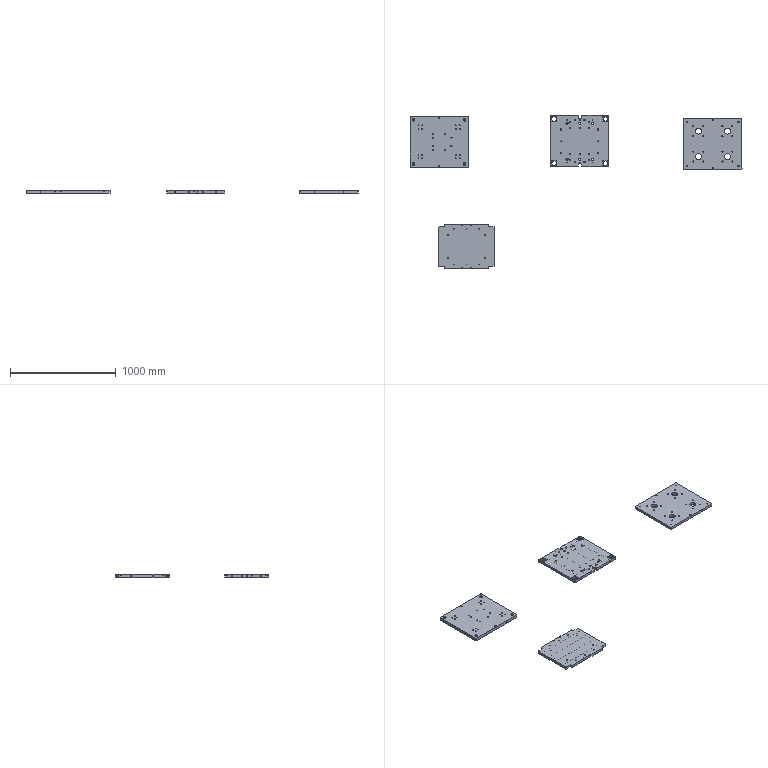NC program | Mastercam | posted with a generic post | part box 3140 x 1452 x 30 mm
Lines 1914 to 2558 of 6493:
N9180 T5 M6
N9190 G0 G90 G17 G54 X-192.57 Y156. A0. S6000 M3
N9200 G43 H5 Z50. M8
N9210 Z1.2
N9220 G1 Z.2 F600.
N9230 G3 X-194.5 Y157.93 Z.1 I-1.93 J0. F2000.
N9240 X-196.43 Y156. Z0. I0. J-1.93
N9250 X-194.5 Y154.07 Z-.1 I1.93 J0.
N9260 X-192.57 Y156. Z-.2 I0. J1.93
N9270 X-194.5 Y157.93 Z-.3 I-1.93 J0.
N9280 X-196.43 Y156. Z-.4 I0. J-1.93
N9290 X-194.5 Y154.07 Z-.5 I1.93 J0.
N9300 X-192.57 Y156. Z-.6 I0. J1.93
N9310 X-194.5 Y157.93 Z-.7 I-1.93 J0.
N9320 X-196.43 Y156. Z-.8 I0. J-1.93
N9330 X-194.5 Y154.07 Z-.9 I1.93 J0.
N9340 X-192.57 Y156. Z-1. I0. J1.93
N9350 X-194.5 Y157.93 Z-1.1 I-1.93 J0.
N9360 X-196.43 Y156. Z-1.2 I0. J-1.93
N9370 X-194.5 Y154.07 Z-1.3 I1.93 J0.
N9380 X-192.57 Y156. Z-1.4 I0. J1.93
N9390 X-194.5 Y157.93 Z-1.5 I-1.93 J0.
N9400 X-196.43 Y156. Z-1.6 I0. J-1.93
N9410 X-194.5 Y154.07 Z-1.7 I1.93 J0.
N9420 X-192.57 Y156. Z-1.8 I0. J1.93
N9430 X-194.5 Y157.93 Z-1.9 I-1.93 J0.
N9440 X-196.43 Y156. Z-2. I0. J-1.93
N9450 X-194.5 Y154.07 Z-2.1 I1.93 J0.
N9460 X-192.57 Y156. Z-2.2 I0. J1.93
N9470 X-194.5 Y157.93 Z-2.3 I-1.93 J0.
N9480 X-196.43 Y156. Z-2.4 I0. J-1.93
N9490 X-194.5 Y154.07 Z-2.5 I1.93 J0.
N9500 X-192.57 Y156. Z-2.6 I0. J1.93
N9510 X-194.5 Y157.93 Z-2.7 I-1.93 J0.
N9520 X-196.43 Y156. Z-2.8 I0. J-1.93
N9530 X-194.5 Y154.07 Z-2.9 I1.93 J0.
N9540 X-192.57 Y156. Z-3. I0. J1.93
N9550 X-194.5 Y157.93 Z-3.1 I-1.93 J0.
N9560 X-196.43 Y156. Z-3.2 I0. J-1.93
N9570 X-194.5 Y154.07 Z-3.3 I1.93 J0.
N9580 X-192.57 Y156. Z-3.4 I0. J1.93
N9590 X-194.5 Y157.93 Z-3.5 I-1.93 J0.
N9600 X-196.43 Y156. Z-3.6 I0. J-1.93
N9610 X-194.5 Y154.07 Z-3.7 I1.93 J0.
N9620 X-192.57 Y156. Z-3.8 I0. J1.93
N9630 X-194.5 Y157.93 Z-3.9 I-1.93 J0.
N9640 X-196.43 Y156. Z-4. I0. J-1.93
N9650 X-194.5 Y154.07 Z-4.1 I1.93 J0.
N9660 X-192.57 Y156. Z-4.2 I0. J1.93
N9670 X-194.5 Y157.93 Z-4.3 I-1.93 J0.
N9680 X-196.43 Y156. Z-4.4 I0. J-1.93
N9690 X-194.5 Y154.07 Z-4.5 I1.93 J0.
N9700 X-192.57 Y156. Z-4.6 I0. J1.93
N9710 X-194.5 Y157.93 Z-4.7 I-1.93 J0.
N9720 X-196.43 Y156. Z-4.8 I0. J-1.93
N9730 X-194.5 Y154.07 Z-4.9 I1.93 J0.
N9740 X-192.57 Y156. Z-5. I0. J1.93
N9750 X-194.5 Y157.93 Z-5.1 I-1.93 J0.
N9760 X-196.43 Y156. Z-5.2 I0. J-1.93
N9770 X-194.5 Y154.07 Z-5.3 I1.93 J0.
N9780 X-192.57 Y156. Z-5.4 I0. J1.93
N9790 X-194.5 Y157.93 Z-5.5 I-1.93 J0.
N9800 X-196.43 Y156. Z-5.6 I0. J-1.93
N9810 X-194.5 Y154.07 Z-5.7 I1.93 J0.
N9820 X-192.57 Y156. Z-5.8 I0. J1.93
N9830 X-194.5 Y157.93 Z-5.9 I-1.93 J0.
N9840 X-196.43 Y156. Z-6. I0. J-1.93
N9850 X-194.5 Y154.07 Z-6.1 I1.93 J0.
N9860 X-192.57 Y156. Z-6.2 I0. J1.93
N9870 X-194.5 Y157.93 Z-6.3 I-1.93 J0.
N9880 X-196.43 Y156. Z-6.4 I0. J-1.93
N9890 X-194.5 Y154.07 Z-6.5 I1.93 J0.
N9900 X-192.57 Y156. Z-6.6 I0. J1.93
N9910 X-194.5 Y157.93 Z-6.7 I-1.93 J0.
N9920 X-196.43 Y156. Z-6.8 I0. J-1.93
N9930 X-194.5 Y154.07 Z-6.9 I1.93 J0.
N9940 X-192.57 Y156. Z-7. I0. J1.93
N9950 X-194.5 Y157.93 Z-7.1 I-1.93 J0.
N9960 X-196.43 Y156. Z-7.2 I0. J-1.93
N9970 X-194.5 Y154.07 Z-7.3 I1.93 J0.
N9980 X-192.57 Y156. Z-7.4 I0. J1.93
N9990 X-194.5 Y157.93 Z-7.5 I-1.93 J0.
N100 X-196.43 Y156. Z-7.6 I0. J-1.93
N110 X-194.5 Y154.07 Z-7.7 I1.93 J0.
N120 X-192.57 Y156. Z-7.8 I0. J1.93
N130 X-194.5 Y157.93 Z-7.9 I-1.93 J0.
N140 X-196.43 Y156. Z-8. I0. J-1.93
N150 X-194.5 Y154.07 Z-8.1 I1.93 J0.
N160 X-192.57 Y156. Z-8.2 I0. J1.93
N170 X-194.5 Y157.93 Z-8.3 I-1.93 J0.
N180 X-196.43 Y156. Z-8.4 I0. J-1.93
N190 X-194.5 Y154.07 Z-8.5 I1.93 J0.
N200 X-192.57 Y156. Z-8.6 I0. J1.93
N210 X-194.5 Y157.93 Z-8.7 I-1.93 J0.
N220 X-196.43 Y156. Z-8.8 I0. J-1.93
N230 X-194.5 Y154.07 Z-8.9 I1.93 J0.
N240 X-192.57 Y156. Z-9. I0. J1.93
N250 X-194.5 Y157.93 Z-9.1 I-1.93 J0.
N260 X-196.43 Y156. Z-9.2 I0. J-1.93
N270 X-194.5 Y154.07 Z-9.3 I1.93 J0.
N280 X-192.57 Y156. Z-9.4 I0. J1.93
N290 X-194.5 Y157.93 Z-9.5 I-1.93 J0.
N300 X-196.43 Y156. Z-9.6 I0. J-1.93
N310 X-194.5 Y154.07 Z-9.7 I1.93 J0.
N320 X-192.57 Y156. Z-9.8 I0. J1.93
N330 X-194.5 Y157.93 Z-9.9 I-1.93 J0.
N340 X-196.43 Y156. Z-10. I0. J-1.93
N350 X-194.5 Y154.07 Z-10.1 I1.93 J0.
N360 X-192.57 Y156. Z-10.2 I0. J1.93
N370 X-194.5 Y157.93 Z-10.3 I-1.93 J0.
N380 X-196.43 Y156. Z-10.4 I0. J-1.93
N390 X-194.5 Y154.07 Z-10.5 I1.93 J0.
N400 X-192.57 Y156. Z-10.6 I0. J1.93
N410 X-194.5 Y157.93 Z-10.7 I-1.93 J0.
N420 X-196.43 Y156. Z-10.8 I0. J-1.93
N430 X-194.5 Y154.07 Z-10.9 I1.93 J0.
N440 X-192.57 Y156. Z-11. I0. J1.93
N450 X-194.5 Y157.93 Z-11.1 I-1.93 J0.
N460 X-196.43 Y156. Z-11.2 I0. J-1.93
N470 X-194.5 Y154.07 Z-11.3 I1.93 J0.
N480 X-192.57 Y156. Z-11.4 I0. J1.93
N490 X-194.5 Y157.93 Z-11.5 I-1.93 J0.
N500 X-196.43 Y156. Z-11.6 I0. J-1.93
N510 X-194.5 Y154.07 Z-11.7 I1.93 J0.
N520 X-192.57 Y156. Z-11.8 I0. J1.93
N530 X-194.5 Y157.93 Z-11.9 I-1.93 J0.
N540 X-196.43 Y156. Z-12. I0. J-1.93
N550 X-194.5 Y154.07 Z-12.1 I1.93 J0.
N560 X-192.57 Y156. Z-12.2 I0. J1.93
N570 X-194.5 Y157.93 Z-12.3 I-1.93 J0.
N580 X-196.43 Y156. Z-12.4 I0. J-1.93
N590 X-194.5 Y154.07 Z-12.5 I1.93 J0.
N600 X-192.57 Y156. Z-12.6 I0. J1.93
N610 X-194.5 Y157.93 Z-12.7 I-1.93 J0.
N620 X-196.43 Y156. Z-12.8 I0. J-1.93
N630 X-194.5 Y154.07 Z-12.9 I1.93 J0.
N640 X-192.57 Y156. Z-13. I0. J1.93
N650 X-194.5 Y157.93 Z-13.1 I-1.93 J0.
N660 X-196.43 Y156. Z-13.2 I0. J-1.93
N670 X-194.5 Y154.07 Z-13.3 I1.93 J0.
N680 X-192.57 Y156. Z-13.4 I0. J1.93
N690 X-194.5 Y157.93 Z-13.5 I-1.93 J0.
N700 X-196.43 Y156. Z-13.6 I0. J-1.93
N710 X-194.5 Y154.07 Z-13.7 I1.93 J0.
N720 X-192.57 Y156. Z-13.8 I0. J1.93
N730 X-194.5 Y157.93 Z-13.9 I-1.93 J0.
N740 X-195.865 Y157.365 Z-13.95 I0. J-1.93
N750 X-196.43 Y156. I1.365 J-1.365
N760 X-194.5 Y154.07 I1.93 J0.
N770 X-192.57 Y156. I0. J1.93
N780 X-194.5 Y157.93 I-1.93 J0.
N790 X-196.169 Y156.97 I0. J-1.93
N800 G0 Z50.
N810 X-192.57 Y124.
N820 Z1.2
N830 G1 Z.2 F600.
N840 G3 X-194.5 Y125.93 Z.1 I-1.93 J0. F2000.
N850 X-196.43 Y124. Z0. I0. J-1.93
N860 X-194.5 Y122.07 Z-.1 I1.93 J0.
N870 X-192.57 Y124. Z-.2 I0. J1.93
N880 X-194.5 Y125.93 Z-.3 I-1.93 J0.
N890 X-196.43 Y124. Z-.4 I0. J-1.93
N900 X-194.5 Y122.07 Z-.5 I1.93 J0.
N910 X-192.57 Y124. Z-.6 I0. J1.93
N920 X-194.5 Y125.93 Z-.7 I-1.93 J0.
N930 X-196.43 Y124. Z-.8 I0. J-1.93
N940 X-194.5 Y122.07 Z-.9 I1.93 J0.
N950 X-192.57 Y124. Z-1. I0. J1.93
N960 X-194.5 Y125.93 Z-1.1 I-1.93 J0.
N970 X-196.43 Y124. Z-1.2 I0. J-1.93
N980 X-194.5 Y122.07 Z-1.3 I1.93 J0.
N990 X-192.57 Y124. Z-1.4 I0. J1.93
N1000 X-194.5 Y125.93 Z-1.5 I-1.93 J0.
N1010 X-196.43 Y124. Z-1.6 I0. J-1.93
N1020 X-194.5 Y122.07 Z-1.7 I1.93 J0.
N1030 X-192.57 Y124. Z-1.8 I0. J1.93
N1040 X-194.5 Y125.93 Z-1.9 I-1.93 J0.
N1050 X-196.43 Y124. Z-2. I0. J-1.93
N1060 X-194.5 Y122.07 Z-2.1 I1.93 J0.
N1070 X-192.57 Y124. Z-2.2 I0. J1.93
N1080 X-194.5 Y125.93 Z-2.3 I-1.93 J0.
N1090 X-196.43 Y124. Z-2.4 I0. J-1.93
N1100 X-194.5 Y122.07 Z-2.5 I1.93 J0.
N1110 X-192.57 Y124. Z-2.6 I0. J1.93
N1120 X-194.5 Y125.93 Z-2.7 I-1.93 J0.
N1130 X-196.43 Y124. Z-2.8 I0. J-1.93
N1140 X-194.5 Y122.07 Z-2.9 I1.93 J0.
N1150 X-192.57 Y124. Z-3. I0. J1.93
N1160 X-194.5 Y125.93 Z-3.1 I-1.93 J0.
N1170 X-196.43 Y124. Z-3.2 I0. J-1.93
N1180 X-194.5 Y122.07 Z-3.3 I1.93 J0.
N1190 X-192.57 Y124. Z-3.4 I0. J1.93
N1200 X-194.5 Y125.93 Z-3.5 I-1.93 J0.
N1210 X-196.43 Y124. Z-3.6 I0. J-1.93
N1220 X-194.5 Y122.07 Z-3.7 I1.93 J0.
N1230 X-192.57 Y124. Z-3.8 I0. J1.93
N1240 X-194.5 Y125.93 Z-3.9 I-1.93 J0.
N1250 X-196.43 Y124. Z-4. I0. J-1.93
N1260 X-194.5 Y122.07 Z-4.1 I1.93 J0.
N1270 X-192.57 Y124. Z-4.2 I0. J1.93
N1280 X-194.5 Y125.93 Z-4.3 I-1.93 J0.
N1290 X-196.43 Y124. Z-4.4 I0. J-1.93
N1300 X-194.5 Y122.07 Z-4.5 I1.93 J0.
N1310 X-192.57 Y124. Z-4.6 I0. J1.93
N1320 X-194.5 Y125.93 Z-4.7 I-1.93 J0.
N1330 X-196.43 Y124. Z-4.8 I0. J-1.93
N1340 X-194.5 Y122.07 Z-4.9 I1.93 J0.
N1350 X-192.57 Y124. Z-5. I0. J1.93
N1360 X-194.5 Y125.93 Z-5.1 I-1.93 J0.
N1370 X-196.43 Y124. Z-5.2 I0. J-1.93
N1380 X-194.5 Y122.07 Z-5.3 I1.93 J0.
N1390 X-192.57 Y124. Z-5.4 I0. J1.93
N1400 X-194.5 Y125.93 Z-5.5 I-1.93 J0.
N1410 X-196.43 Y124. Z-5.6 I0. J-1.93
N1420 X-194.5 Y122.07 Z-5.7 I1.93 J0.
N1430 X-192.57 Y124. Z-5.8 I0. J1.93
N1440 X-194.5 Y125.93 Z-5.9 I-1.93 J0.
N1450 X-196.43 Y124. Z-6. I0. J-1.93
N1460 X-194.5 Y122.07 Z-6.1 I1.93 J0.
N1470 X-192.57 Y124. Z-6.2 I0. J1.93
N1480 X-194.5 Y125.93 Z-6.3 I-1.93 J0.
N1490 X-196.43 Y124. Z-6.4 I0. J-1.93
N1500 X-194.5 Y122.07 Z-6.5 I1.93 J0.
N1510 X-192.57 Y124. Z-6.6 I0. J1.93
N1520 X-194.5 Y125.93 Z-6.7 I-1.93 J0.
N1530 X-196.43 Y124. Z-6.8 I0. J-1.93
N1540 X-194.5 Y122.07 Z-6.9 I1.93 J0.
N1550 X-192.57 Y124. Z-7. I0. J1.93
N1560 X-194.5 Y125.93 Z-7.1 I-1.93 J0.
N1570 X-196.43 Y124. Z-7.2 I0. J-1.93
N1580 X-194.5 Y122.07 Z-7.3 I1.93 J0.
N1590 X-192.57 Y124. Z-7.4 I0. J1.93
N1600 X-194.5 Y125.93 Z-7.5 I-1.93 J0.
N1610 X-196.43 Y124. Z-7.6 I0. J-1.93
N1620 X-194.5 Y122.07 Z-7.7 I1.93 J0.
N1630 X-192.57 Y124. Z-7.8 I0. J1.93
N1640 X-194.5 Y125.93 Z-7.9 I-1.93 J0.
N1650 X-196.43 Y124. Z-8. I0. J-1.93
N1660 X-194.5 Y122.07 Z-8.1 I1.93 J0.
N1670 X-192.57 Y124. Z-8.2 I0. J1.93
N1680 X-194.5 Y125.93 Z-8.3 I-1.93 J0.
N1690 X-196.43 Y124. Z-8.4 I0. J-1.93
N1700 X-194.5 Y122.07 Z-8.5 I1.93 J0.
N1710 X-192.57 Y124. Z-8.6 I0. J1.93
N1720 X-194.5 Y125.93 Z-8.7 I-1.93 J0.
N1730 X-196.43 Y124. Z-8.8 I0. J-1.93
N1740 X-194.5 Y122.07 Z-8.9 I1.93 J0.
N1750 X-192.57 Y124. Z-9. I0. J1.93
N1760 X-194.5 Y125.93 Z-9.1 I-1.93 J0.
N1770 X-196.43 Y124. Z-9.2 I0. J-1.93
N1780 X-194.5 Y122.07 Z-9.3 I1.93 J0.
N1790 X-192.57 Y124. Z-9.4 I0. J1.93
N1800 X-194.5 Y125.93 Z-9.5 I-1.93 J0.
N1810 X-196.43 Y124. Z-9.6 I0. J-1.93
N1820 X-194.5 Y122.07 Z-9.7 I1.93 J0.
N1830 X-192.57 Y124. Z-9.8 I0. J1.93
N1840 X-194.5 Y125.93 Z-9.9 I-1.93 J0.
N1850 X-196.43 Y124. Z-10. I0. J-1.93
N1860 X-194.5 Y122.07 Z-10.1 I1.93 J0.
N1870 X-192.57 Y124. Z-10.2 I0. J1.93
N1880 X-194.5 Y125.93 Z-10.3 I-1.93 J0.
N1890 X-196.43 Y124. Z-10.4 I0. J-1.93
N1900 X-194.5 Y122.07 Z-10.5 I1.93 J0.
N1910 X-192.57 Y124. Z-10.6 I0. J1.93
N1920 X-194.5 Y125.93 Z-10.7 I-1.93 J0.
N1930 X-196.43 Y124. Z-10.8 I0. J-1.93
N1940 X-194.5 Y122.07 Z-10.9 I1.93 J0.
N1950 X-192.57 Y124. Z-11. I0. J1.93
N1960 X-194.5 Y125.93 Z-11.1 I-1.93 J0.
N1970 X-196.43 Y124. Z-11.2 I0. J-1.93
N1980 X-194.5 Y122.07 Z-11.3 I1.93 J0.
N1990 X-192.57 Y124. Z-11.4 I0. J1.93
N2000 X-194.5 Y125.93 Z-11.5 I-1.93 J0.
N2010 X-196.43 Y124. Z-11.6 I0. J-1.93
N2020 X-194.5 Y122.07 Z-11.7 I1.93 J0.
N2030 X-192.57 Y124. Z-11.8 I0. J1.93
N2040 X-194.5 Y125.93 Z-11.9 I-1.93 J0.
N2050 X-196.43 Y124. Z-12. I0. J-1.93
N2060 X-194.5 Y122.07 Z-12.1 I1.93 J0.
N2070 X-192.57 Y124. Z-12.2 I0. J1.93
N2080 X-194.5 Y125.93 Z-12.3 I-1.93 J0.
N2090 X-196.43 Y124. Z-12.4 I0. J-1.93
N2100 X-194.5 Y122.07 Z-12.5 I1.93 J0.
N2110 X-192.57 Y124. Z-12.6 I0. J1.93
N2120 X-194.5 Y125.93 Z-12.7 I-1.93 J0.
N2130 X-196.43 Y124. Z-12.8 I0. J-1.93
N2140 X-194.5 Y122.07 Z-12.9 I1.93 J0.
N2150 X-192.57 Y124. Z-13. I0. J1.93
N2160 X-194.5 Y125.93 Z-13.1 I-1.93 J0.
N2170 X-196.43 Y124. Z-13.2 I0. J-1.93
N2180 X-194.5 Y122.07 Z-13.3 I1.93 J0.
N2190 X-192.57 Y124. Z-13.4 I0. J1.93
N2200 X-194.5 Y125.93 Z-13.5 I-1.93 J0.
N2210 X-196.43 Y124. Z-13.6 I0. J-1.93
N2220 X-194.5 Y122.07 Z-13.7 I1.93 J0.
N2230 X-192.57 Y124. Z-13.8 I0. J1.93
N2240 X-194.5 Y125.93 Z-13.9 I-1.93 J0.
N2250 X-195.865 Y125.365 Z-13.95 I0. J-1.93
N2260 X-196.43 Y124. I1.365 J-1.365
N2270 X-194.5 Y122.07 I1.93 J0.
N2280 X-192.57 Y124. I0. J1.93
N2290 X-194.5 Y125.93 I-1.93 J0.
N2300 X-196.169 Y124.97 I0. J-1.93
N2310 G0 Z50.
N2320 X-156.57 Y156.
N2330 Z1.2
N2340 G1 Z.2 F600.
N2350 G3 X-158.5 Y157.93 Z.1 I-1.93 J0. F2000.
N2360 X-160.43 Y156. Z0. I0. J-1.93
N2370 X-158.5 Y154.07 Z-.1 I1.93 J0.
N2380 X-156.57 Y156. Z-.2 I0. J1.93
N2390 X-158.5 Y157.93 Z-.3 I-1.93 J0.
N2400 X-160.43 Y156. Z-.4 I0. J-1.93
N2410 X-158.5 Y154.07 Z-.5 I1.93 J0.
N2420 X-156.57 Y156. Z-.6 I0. J1.93
N2430 X-158.5 Y157.93 Z-.7 I-1.93 J0.
N2440 X-160.43 Y156. Z-.8 I0. J-1.93
N2450 X-158.5 Y154.07 Z-.9 I1.93 J0.
N2460 X-156.57 Y156. Z-1. I0. J1.93
N2470 X-158.5 Y157.93 Z-1.1 I-1.93 J0.
N2480 X-160.43 Y156. Z-1.2 I0. J-1.93
N2490 X-158.5 Y154.07 Z-1.3 I1.93 J0.
N2500 X-156.57 Y156. Z-1.4 I0. J1.93
N2510 X-158.5 Y157.93 Z-1.5 I-1.93 J0.
N2520 X-160.43 Y156. Z-1.6 I0. J-1.93
N2530 X-158.5 Y154.07 Z-1.7 I1.93 J0.
N2540 X-156.57 Y156. Z-1.8 I0. J1.93
N2550 X-158.5 Y157.93 Z-1.9 I-1.93 J0.
N2560 X-160.43 Y156. Z-2. I0. J-1.93
N2570 X-158.5 Y154.07 Z-2.1 I1.93 J0.
N2580 X-156.57 Y156. Z-2.2 I0. J1.93
N2590 X-158.5 Y157.93 Z-2.3 I-1.93 J0.
N2600 X-160.43 Y156. Z-2.4 I0. J-1.93
N2610 X-158.5 Y154.07 Z-2.5 I1.93 J0.
N2620 X-156.57 Y156. Z-2.6 I0. J1.93
N2630 X-158.5 Y157.93 Z-2.7 I-1.93 J0.
N2640 X-160.43 Y156. Z-2.8 I0. J-1.93
N2650 X-158.5 Y154.07 Z-2.9 I1.93 J0.
N2660 X-156.57 Y156. Z-3. I0. J1.93
N2670 X-158.5 Y157.93 Z-3.1 I-1.93 J0.
N2680 X-160.43 Y156. Z-3.2 I0. J-1.93
N2690 X-158.5 Y154.07 Z-3.3 I1.93 J0.
N2700 X-156.57 Y156. Z-3.4 I0. J1.93
N2710 X-158.5 Y157.93 Z-3.5 I-1.93 J0.
N2720 X-160.43 Y156. Z-3.6 I0. J-1.93
N2730 X-158.5 Y154.07 Z-3.7 I1.93 J0.
N2740 X-156.57 Y156. Z-3.8 I0. J1.93
N2750 X-158.5 Y157.93 Z-3.9 I-1.93 J0.
N2760 X-160.43 Y156. Z-4. I0. J-1.93
N2770 X-158.5 Y154.07 Z-4.1 I1.93 J0.
N2780 X-156.57 Y156. Z-4.2 I0. J1.93
N2790 X-158.5 Y157.93 Z-4.3 I-1.93 J0.
N2800 X-160.43 Y156. Z-4.4 I0. J-1.93
N2810 X-158.5 Y154.07 Z-4.5 I1.93 J0.
N2820 X-156.57 Y156. Z-4.6 I0. J1.93
N2830 X-158.5 Y157.93 Z-4.7 I-1.93 J0.
N2840 X-160.43 Y156. Z-4.8 I0. J-1.93
N2850 X-158.5 Y154.07 Z-4.9 I1.93 J0.
N2860 X-156.57 Y156. Z-5. I0. J1.93
N2870 X-158.5 Y157.93 Z-5.1 I-1.93 J0.
N2880 X-160.43 Y156. Z-5.2 I0. J-1.93
N2890 X-158.5 Y154.07 Z-5.3 I1.93 J0.
N2900 X-156.57 Y156. Z-5.4 I0. J1.93
N2910 X-158.5 Y157.93 Z-5.5 I-1.93 J0.
N2920 X-160.43 Y156. Z-5.6 I0. J-1.93
N2930 X-158.5 Y154.07 Z-5.7 I1.93 J0.
N2940 X-156.57 Y156. Z-5.8 I0. J1.93
N2950 X-158.5 Y157.93 Z-5.9 I-1.93 J0.
N2960 X-160.43 Y156. Z-6. I0. J-1.93
N2970 X-158.5 Y154.07 Z-6.1 I1.93 J0.
N2980 X-156.57 Y156. Z-6.2 I0. J1.93
N2990 X-158.5 Y157.93 Z-6.3 I-1.93 J0.
N3000 X-160.43 Y156. Z-6.4 I0. J-1.93
N3010 X-158.5 Y154.07 Z-6.5 I1.93 J0.
N3020 X-156.57 Y156. Z-6.6 I0. J1.93
N3030 X-158.5 Y157.93 Z-6.7 I-1.93 J0.
N3040 X-160.43 Y156. Z-6.8 I0. J-1.93
N3050 X-158.5 Y154.07 Z-6.9 I1.93 J0.
N3060 X-156.57 Y156. Z-7. I0. J1.93
N3070 X-158.5 Y157.93 Z-7.1 I-1.93 J0.
N3080 X-160.43 Y156. Z-7.2 I0. J-1.93
N3090 X-158.5 Y154.07 Z-7.3 I1.93 J0.
N3100 X-156.57 Y156. Z-7.4 I0. J1.93
N3110 X-158.5 Y157.93 Z-7.5 I-1.93 J0.
N3120 X-160.43 Y156. Z-7.6 I0. J-1.93
N3130 X-158.5 Y154.07 Z-7.7 I1.93 J0.
N3140 X-156.57 Y156. Z-7.8 I0. J1.93
N3150 X-158.5 Y157.93 Z-7.9 I-1.93 J0.
N3160 X-160.43 Y156. Z-8. I0. J-1.93
N3170 X-158.5 Y154.07 Z-8.1 I1.93 J0.
N3180 X-156.57 Y156. Z-8.2 I0. J1.93
N3190 X-158.5 Y157.93 Z-8.3 I-1.93 J0.
N3200 X-160.43 Y156. Z-8.4 I0. J-1.93
N3210 X-158.5 Y154.07 Z-8.5 I1.93 J0.
N3220 X-156.57 Y156. Z-8.6 I0. J1.93
N3230 X-158.5 Y157.93 Z-8.7 I-1.93 J0.
N3240 X-160.43 Y156. Z-8.8 I0. J-1.93
N3250 X-158.5 Y154.07 Z-8.9 I1.93 J0.
N3260 X-156.57 Y156. Z-9. I0. J1.93
N3270 X-158.5 Y157.93 Z-9.1 I-1.93 J0.
N3280 X-160.43 Y156. Z-9.2 I0. J-1.93
N3290 X-158.5 Y154.07 Z-9.3 I1.93 J0.
N3300 X-156.57 Y156. Z-9.4 I0. J1.93
N3310 X-158.5 Y157.93 Z-9.5 I-1.93 J0.
N3320 X-160.43 Y156. Z-9.6 I0. J-1.93
N3330 X-158.5 Y154.07 Z-9.7 I1.93 J0.
N3340 X-156.57 Y156. Z-9.8 I0. J1.93
N3350 X-158.5 Y157.93 Z-9.9 I-1.93 J0.
N3360 X-160.43 Y156. Z-10. I0. J-1.93
N3370 X-158.5 Y154.07 Z-10.1 I1.93 J0.
N3380 X-156.57 Y156. Z-10.2 I0. J1.93
N3390 X-158.5 Y157.93 Z-10.3 I-1.93 J0.
N3400 X-160.43 Y156. Z-10.4 I0. J-1.93
N3410 X-158.5 Y154.07 Z-10.5 I1.93 J0.
N3420 X-156.57 Y156. Z-10.6 I0. J1.93
N3430 X-158.5 Y157.93 Z-10.7 I-1.93 J0.
N3440 X-160.43 Y156. Z-10.8 I0. J-1.93
N3450 X-158.5 Y154.07 Z-10.9 I1.93 J0.
N3460 X-156.57 Y156. Z-11. I0. J1.93
N3470 X-158.5 Y157.93 Z-11.1 I-1.93 J0.
N3480 X-160.43 Y156. Z-11.2 I0. J-1.93
N3490 X-158.5 Y154.07 Z-11.3 I1.93 J0.
N3500 X-156.57 Y156. Z-11.4 I0. J1.93
N3510 X-158.5 Y157.93 Z-11.5 I-1.93 J0.
N3520 X-160.43 Y156. Z-11.6 I0. J-1.93
N3530 X-158.5 Y154.07 Z-11.7 I1.93 J0.
N3540 X-156.57 Y156. Z-11.8 I0. J1.93
N3550 X-158.5 Y157.93 Z-11.9 I-1.93 J0.
N3560 X-160.43 Y156. Z-12. I0. J-1.93
N3570 X-158.5 Y154.07 Z-12.1 I1.93 J0.
N3580 X-156.57 Y156. Z-12.2 I0. J1.93
N3590 X-158.5 Y157.93 Z-12.3 I-1.93 J0.
N3600 X-160.43 Y156. Z-12.4 I0. J-1.93
N3610 X-158.5 Y154.07 Z-12.5 I1.93 J0.
N3620 X-156.57 Y156. Z-12.6 I0. J1.93
N3630 X-158.5 Y157.93 Z-12.7 I-1.93 J0.
N3640 X-160.43 Y156. Z-12.8 I0. J-1.93
N3650 X-158.5 Y154.07 Z-12.9 I1.93 J0.
N3660 X-156.57 Y156. Z-13. I0. J1.93
N3670 X-158.5 Y157.93 Z-13.1 I-1.93 J0.
N3680 X-160.43 Y156. Z-13.2 I0. J-1.93
N3690 X-158.5 Y154.07 Z-13.3 I1.93 J0.
N3700 X-156.57 Y156. Z-13.4 I0. J1.93
N3710 X-158.5 Y157.93 Z-13.5 I-1.93 J0.
N3720 X-160.43 Y156. Z-13.6 I0. J-1.93
N3730 X-158.5 Y154.07 Z-13.7 I1.93 J0.
N3740 X-156.57 Y156. Z-13.8 I0. J1.93
N3750 X-158.5 Y157.93 Z-13.9 I-1.93 J0.
N3760 X-159.865 Y157.365 Z-13.95 I0. J-1.93
N3770 X-160.43 Y156. I1.365 J-1.365
N3780 X-158.5 Y154.07 I1.93 J0.
N3790 X-156.57 Y156. I0. J1.93
N3800 X-158.5 Y157.93 I-1.93 J0.
N3810 X-160.169 Y156.97 I0. J-1.93
N3820 G0 Z50.
N3830 X-156.57 Y124.
N3840 Z1.2
N3850 G1 Z.2 F600.
N3860 G3 X-158.5 Y125.93 Z.1 I-1.93 J0. F2000.
N3870 X-160.43 Y124. Z0. I0. J-1.93
N3880 X-158.5 Y122.07 Z-.1 I1.93 J0.
N3890 X-156.57 Y124. Z-.2 I0. J1.93
N3900 X-158.5 Y125.93 Z-.3 I-1.93 J0.
N3910 X-160.43 Y124. Z-.4 I0. J-1.93
N3920 X-158.5 Y122.07 Z-.5 I1.93 J0.
N3930 X-156.57 Y124. Z-.6 I0. J1.93
N3940 X-158.5 Y125.93 Z-.7 I-1.93 J0.
N3950 X-160.43 Y124. Z-.8 I0. J-1.93
N3960 X-158.5 Y122.07 Z-.9 I1.93 J0.
N3970 X-156.57 Y124. Z-1. I0. J1.93
N3980 X-158.5 Y125.93 Z-1.1 I-1.93 J0.
N3990 X-160.43 Y124. Z-1.2 I0. J-1.93
N4000 X-158.5 Y122.07 Z-1.3 I1.93 J0.
N4010 X-156.57 Y124. Z-1.4 I0. J1.93
N4020 X-158.5 Y125.93 Z-1.5 I-1.93 J0.
N4030 X-160.43 Y124. Z-1.6 I0. J-1.93
N4040 X-158.5 Y122.07 Z-1.7 I1.93 J0.
N4050 X-156.57 Y124. Z-1.8 I0. J1.93
N4060 X-158.5 Y125.93 Z-1.9 I-1.93 J0.
N4070 X-160.43 Y124. Z-2. I0. J-1.93
N4080 X-158.5 Y122.07 Z-2.1 I1.93 J0.
N4090 X-156.57 Y124. Z-2.2 I0. J1.93
N4100 X-158.5 Y125.93 Z-2.3 I-1.93 J0.
N4110 X-160.43 Y124. Z-2.4 I0. J-1.93
N4120 X-158.5 Y122.07 Z-2.5 I1.93 J0.
N4130 X-156.57 Y124. Z-2.6 I0. J1.93
N4140 X-158.5 Y125.93 Z-2.7 I-1.93 J0.
N4150 X-160.43 Y124. Z-2.8 I0. J-1.93
N4160 X-158.5 Y122.07 Z-2.9 I1.93 J0.
N4170 X-156.57 Y124. Z-3. I0. J1.93
N4180 X-158.5 Y125.93 Z-3.1 I-1.93 J0.
N4190 X-160.43 Y124. Z-3.2 I0. J-1.93
N4200 X-158.5 Y122.07 Z-3.3 I1.93 J0.
N4210 X-156.57 Y124. Z-3.4 I0. J1.93
N4220 X-158.5 Y125.93 Z-3.5 I-1.93 J0.
N4230 X-160.43 Y124. Z-3.6 I0. J-1.93
N4240 X-158.5 Y122.07 Z-3.7 I1.93 J0.
N4250 X-156.57 Y124. Z-3.8 I0. J1.93
N4260 X-158.5 Y125.93 Z-3.9 I-1.93 J0.
N4270 X-160.43 Y124. Z-4. I0. J-1.93
N4280 X-158.5 Y122.07 Z-4.1 I1.93 J0.
N4290 X-156.57 Y124. Z-4.2 I0. J1.93
N4300 X-158.5 Y125.93 Z-4.3 I-1.93 J0.
N4310 X-160.43 Y124. Z-4.4 I0. J-1.93
N4320 X-158.5 Y122.07 Z-4.5 I1.93 J0.
N4330 X-156.57 Y124. Z-4.6 I0. J1.93
N4340 X-158.5 Y125.93 Z-4.7 I-1.93 J0.
N4350 X-160.43 Y124. Z-4.8 I0. J-1.93
N4360 X-158.5 Y122.07 Z-4.9 I1.93 J0.
N4370 X-156.57 Y124. Z-5. I0. J1.93
N4380 X-158.5 Y125.93 Z-5.1 I-1.93 J0.
N4390 X-160.43 Y124. Z-5.2 I0. J-1.93
N4400 X-158.5 Y122.07 Z-5.3 I1.93 J0.
N4410 X-156.57 Y124. Z-5.4 I0. J1.93
N4420 X-158.5 Y125.93 Z-5.5 I-1.93 J0.
N4430 X-160.43 Y124. Z-5.6 I0. J-1.93
N4440 X-158.5 Y122.07 Z-5.7 I1.93 J0.
N4450 X-156.57 Y124. Z-5.8 I0. J1.93
N4460 X-158.5 Y125.93 Z-5.9 I-1.93 J0.
N4470 X-160.43 Y124. Z-6. I0. J-1.93
N4480 X-158.5 Y122.07 Z-6.1 I1.93 J0.
N4490 X-156.57 Y124. Z-6.2 I0. J1.93
N4500 X-158.5 Y125.93 Z-6.3 I-1.93 J0.
N4510 X-160.43 Y124. Z-6.4 I0. J-1.93
N4520 X-158.5 Y122.07 Z-6.5 I1.93 J0.
N4530 X-156.57 Y124. Z-6.6 I0. J1.93
N4540 X-158.5 Y125.93 Z-6.7 I-1.93 J0.
N4550 X-160.43 Y124. Z-6.8 I0. J-1.93
N4560 X-158.5 Y122.07 Z-6.9 I1.93 J0.
N4570 X-156.57 Y124. Z-7. I0. J1.93
N4580 X-158.5 Y125.93 Z-7.1 I-1.93 J0.
N4590 X-160.43 Y124. Z-7.2 I0. J-1.93
N4600 X-158.5 Y122.07 Z-7.3 I1.93 J0.
N4610 X-156.57 Y124. Z-7.4 I0. J1.93
N4620 X-158.5 Y125.93 Z-7.5 I-1.93 J0.
N4630 X-160.43 Y124. Z-7.6 I0. J-1.93
N4640 X-158.5 Y122.07 Z-7.7 I1.93 J0.
N4650 X-156.57 Y124. Z-7.8 I0. J1.93
N4660 X-158.5 Y125.93 Z-7.9 I-1.93 J0.
N4670 X-160.43 Y124. Z-8. I0. J-1.93
N4680 X-158.5 Y122.07 Z-8.1 I1.93 J0.
N4690 X-156.57 Y124. Z-8.2 I0. J1.93
N4700 X-158.5 Y125.93 Z-8.3 I-1.93 J0.
N4710 X-160.43 Y124. Z-8.4 I0. J-1.93
N4720 X-158.5 Y122.07 Z-8.5 I1.93 J0.
N4730 X-156.57 Y124. Z-8.6 I0. J1.93
N4740 X-158.5 Y125.93 Z-8.7 I-1.93 J0.
N4750 X-160.43 Y124. Z-8.8 I0. J-1.93
N4760 X-158.5 Y122.07 Z-8.9 I1.93 J0.
N4770 X-156.57 Y124. Z-9. I0. J1.93
N4780 X-158.5 Y125.93 Z-9.1 I-1.93 J0.
N4790 X-160.43 Y124. Z-9.2 I0. J-1.93
N4800 X-158.5 Y122.07 Z-9.3 I1.93 J0.
N4810 X-156.57 Y124. Z-9.4 I0. J1.93
N4820 X-158.5 Y125.93 Z-9.5 I-1.93 J0.
N4830 X-160.43 Y124. Z-9.6 I0. J-1.93
N4840 X-158.5 Y122.07 Z-9.7 I1.93 J0.
N4850 X-156.57 Y124. Z-9.8 I0. J1.93
N4860 X-158.5 Y125.93 Z-9.9 I-1.93 J0.
N4870 X-160.43 Y124. Z-10. I0. J-1.93
N4880 X-158.5 Y122.07 Z-10.1 I1.93 J0.
N4890 X-156.57 Y124. Z-10.2 I0. J1.93
N4900 X-158.5 Y125.93 Z-10.3 I-1.93 J0.
N4910 X-160.43 Y124. Z-10.4 I0. J-1.93
N4920 X-158.5 Y122.07 Z-10.5 I1.93 J0.
N4930 X-156.57 Y124. Z-10.6 I0. J1.93
N4940 X-158.5 Y125.93 Z-10.7 I-1.93 J0.
N4950 X-160.43 Y124. Z-10.8 I0. J-1.93
N4960 X-158.5 Y122.07 Z-10.9 I1.93 J0.
N4970 X-156.57 Y124. Z-11. I0. J1.93
N4980 X-158.5 Y125.93 Z-11.1 I-1.93 J0.
N4990 X-160.43 Y124. Z-11.2 I0. J-1.93
N5000 X-158.5 Y122.07 Z-11.3 I1.93 J0.
N5010 X-156.57 Y124. Z-11.4 I0. J1.93
N5020 X-158.5 Y125.93 Z-11.5 I-1.93 J0.
N5030 X-160.43 Y124. Z-11.6 I0. J-1.93
N5040 X-158.5 Y122.07 Z-11.7 I1.93 J0.
N5050 X-156.57 Y124. Z-11.8 I0. J1.93
N5060 X-158.5 Y125.93 Z-11.9 I-1.93 J0.
N5070 X-160.43 Y124. Z-12. I0. J-1.93
N5080 X-158.5 Y122.07 Z-12.1 I1.93 J0.
N5090 X-156.57 Y124. Z-12.2 I0. J1.93
N5100 X-158.5 Y125.93 Z-12.3 I-1.93 J0.
N5110 X-160.43 Y124. Z-12.4 I0. J-1.93
N5120 X-158.5 Y122.07 Z-12.5 I1.93 J0.
N5130 X-156.57 Y124. Z-12.6 I0. J1.93
N5140 X-158.5 Y125.93 Z-12.7 I-1.93 J0.
N5150 X-160.43 Y124. Z-12.8 I0. J-1.93
N5160 X-158.5 Y122.07 Z-12.9 I1.93 J0.
N5170 X-156.57 Y124. Z-13. I0. J1.93
N5180 X-158.5 Y125.93 Z-13.1 I-1.93 J0.
N5190 X-160.43 Y124. Z-13.2 I0. J-1.93
N5200 X-158.5 Y122.07 Z-13.3 I1.93 J0.
N5210 X-156.57 Y124. Z-13.4 I0. J1.93
N5220 X-158.5 Y125.93 Z-13.5 I-1.93 J0.
N5230 X-160.43 Y124. Z-13.6 I0. J-1.93
N5240 X-158.5 Y122.07 Z-13.7 I1.93 J0.
N5250 X-156.57 Y124. Z-13.8 I0. J1.93
N5260 X-158.5 Y125.93 Z-13.9 I-1.93 J0.
N5270 X-159.865 Y125.365 Z-13.95 I0. J-1.93
N5280 X-160.43 Y124. I1.365 J-1.365
N5290 X-158.5 Y122.07 I1.93 J0.
N5300 X-156.57 Y124. I0. J1.93
N5310 X-158.5 Y125.93 I-1.93 J0.
N5320 X-160.169 Y124.97 I0. J-1.93
N5330 G0 Z50.
N5340 X160.43 Y156.
N5350 Z1.2
N5360 G1 Z.2 F600.
N5370 G3 X158.5 Y157.93 Z.1 I-1.93 J0. F2000.
N5380 X156.57 Y156. Z0. I0. J-1.93
N5390 X158.5 Y154.07 Z-.1 I1.93 J0.
N5400 X160.43 Y156. Z-.2 I0. J1.93
N5410 X158.5 Y157.93 Z-.3 I-1.93 J0.
N5420 X156.57 Y156. Z-.4 I0. J-1.93
N5430 X158.5 Y154.07 Z-.5 I1.93 J0.
N5440 X160.43 Y156. Z-.6 I0. J1.93
N5450 X158.5 Y157.93 Z-.7 I-1.93 J0.
N5460 X156.57 Y156. Z-.8 I0. J-1.93
N5470 X158.5 Y154.07 Z-.9 I1.93 J0.
N5480 X160.43 Y156. Z-1. I0. J1.93
N5490 X158.5 Y157.93 Z-1.1 I-1.93 J0.
N5500 X156.57 Y156. Z-1.2 I0. J-1.93
N5510 X158.5 Y154.07 Z-1.3 I1.93 J0.
N5520 X160.43 Y156. Z-1.4 I0. J1.93
N5530 X158.5 Y157.93 Z-1.5 I-1.93 J0.
N5540 X156.57 Y156. Z-1.6 I0. J-1.93
N5550 X158.5 Y154.07 Z-1.7 I1.93 J0.
N5560 X160.43 Y156. Z-1.8 I0. J1.93
N5570 X158.5 Y157.93 Z-1.9 I-1.93 J0.
N5580 X156.57 Y156. Z-2. I0. J-1.93
N5590 X158.5 Y154.07 Z-2.1 I1.93 J0.
N5600 X160.43 Y156. Z-2.2 I0. J1.93
N5610 X158.5 Y157.93 Z-2.3 I-1.93 J0.
N5620 X156.57 Y156. Z-2.4 I0. J-1.93
N5630 X158.5 Y154.07 Z-2.5 I1.93 J0.
N5640 X160.43 Y156. Z-2.6 I0. J1.93
N5650 X158.5 Y157.93 Z-2.7 I-1.93 J0.
N5660 X156.57 Y156. Z-2.8 I0. J-1.93
N5670 X158.5 Y154.07 Z-2.9 I1.93 J0.
N5680 X160.43 Y156. Z-3. I0. J1.93
N5690 X158.5 Y157.93 Z-3.1 I-1.93 J0.
N5700 X156.57 Y156. Z-3.2 I0. J-1.93
N5710 X158.5 Y154.07 Z-3.3 I1.93 J0.
N5720 X160.43 Y156. Z-3.4 I0. J1.93